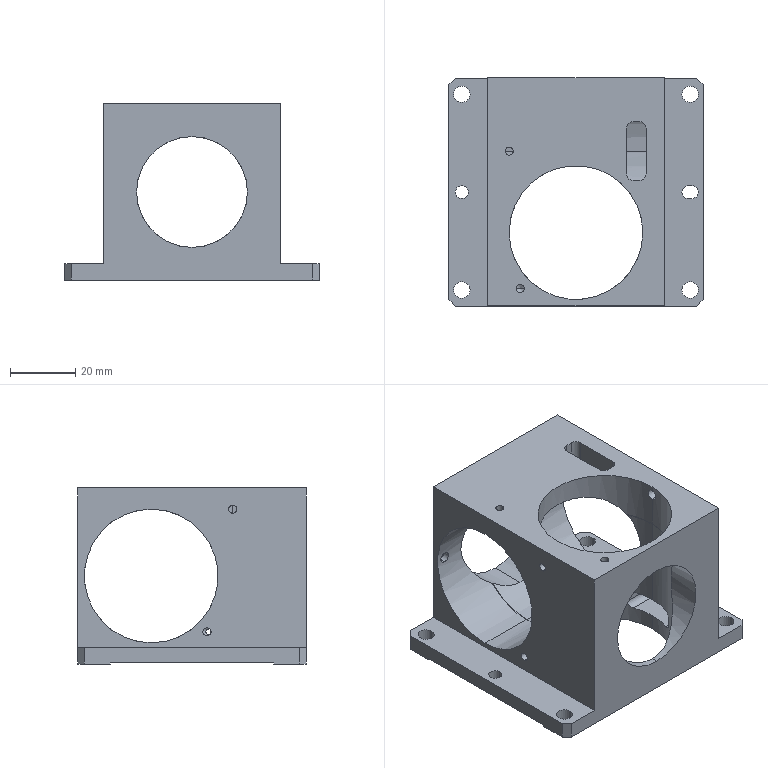NC program | NX | posted with a generic post | part box 78 x 70 x 54 mm
Whole program:
N10 G17 G21 G94 G90
(HOLE_MILLING_COPY , TOOL : D20)
N12 T02 M6
N14 G54
N16 G17 G0 G90 X0. Y0. B0. C0. S9500 M3
N18 G43 Z30. H2
N20 Z0.5
N22 G94 G3 X3.45 Y-3.45 R3.45 F1500.
N24 X6.9 Y0. R3.45
N26 X6.9 Y0. Z0. I-6.9 J0.
N28 X6.9 Y0. Z-0.5 I-6.9 J0.
N30 X6.9 Y0. Z-1. I-6.9 J0.
N32 X6.9 Y0. Z-1.5 I-6.9 J0.
N34 X6.9 Y0. Z-2. I-6.9 J0.
N36 X6.9 Y0. Z-2.5 I-6.9 J0.
N38 X6.9 Y0. Z-3. I-6.9 J0.
N40 X6.9 Y0. Z-3.5 I-6.9 J0.
N42 X6.9 Y0. Z-4. I-6.9 J0.
N44 X6.9 Y0. Z-4.5 I-6.9 J0.
N46 X6.9 Y0. Z-5. I-6.9 J0.
N48 X6.9 Y0. Z-5.5 I-6.9 J0.
N50 X6.9 Y0. Z-6. I-6.9 J0.
N52 X6.9 Y0. Z-6.5 I-6.9 J0.
N54 X6.9 Y0. Z-7. I-6.9 J0.
N56 X6.9 Y0. Z-7.5 I-6.9 J0.
N58 X6.9 Y0. Z-8. I-6.9 J0.
N60 X6.9 Y0. Z-8.5 I-6.9 J0.
N62 X6.9 Y0. Z-9. I-6.9 J0.
N64 X6.9 Y0. Z-9.5 I-6.9 J0.
N66 X6.9 Y0. Z-10. I-6.9 J0.
N68 X6.9 Y0. Z-10.5 I-6.9 J0.
N70 X6.9 Y0. Z-11. I-6.9 J0.
N72 X6.9 Y0. Z-11.5 I-6.9 J0.
N74 X6.9 Y0. Z-12. I-6.9 J0.
N76 X6.9 Y0. Z-12.5 I-6.9 J0.
N78 X6.9 Y0. Z-13. I-6.9 J0.
N80 X6.9 Y0. Z-13.5 I-6.9 J0.
N82 X6.9 Y0. Z-14. I-6.9 J0.
N84 X6.9 Y0. Z-14.5 I-6.9 J0.
N86 X6.9 Y0. Z-15. I-6.9 J0.
N88 X6.9 Y0. Z-15.5 I-6.9 J0.
N90 X6.9 Y0. Z-16. I-6.9 J0.
N92 X6.9 Y0. Z-16.5 I-6.9 J0.
N94 X6.9 Y0. Z-17. I-6.9 J0.
N96 X6.9 Y0. Z-17.5 I-6.9 J0.
N98 X6.9 Y0. Z-18. I-6.9 J0.
N100 X6.9 Y0. Z-18.5 I-6.9 J0.
N102 X6.9 Y0. Z-19. I-6.9 J0.
N104 X6.9 Y0. Z-19.5 I-6.9 J0.
N106 X6.9 Y0. Z-20. I-6.9 J0.
N108 X6.9 Y0. Z-20.5 I-6.9 J0.
N110 X6.9 Y0. Z-21. I-6.9 J0.
N112 X6.9 Y0. Z-21.5 I-6.9 J0.
N114 X6.9 Y0. Z-22. I-6.9 J0.
N116 X6.9 Y0. Z-22.5 I-6.9 J0.
N118 X6.9 Y0. Z-23. I-6.9 J0.
N120 X6.9 Y0. Z-23.5 I-6.9 J0.
N122 X6.9 Y0. Z-24. I-6.9 J0.
N124 X6.9 Y0. Z-24.5 I-6.9 J0.
N126 X6.9 Y0. Z-25. I-6.9 J0.
N128 X6.9 Y0. Z-25.5 I-6.9 J0.
N130 X6.9 Y0. Z-26. I-6.9 J0.
N132 X6.9 Y0. Z-26.5 I-6.9 J0.
N134 X6.9 Y0. Z-27. I-6.9 J0.
N136 X6.9 Y0. Z-27.5 I-6.9 J0.
N138 X6.9 Y0. Z-28. I-6.9 J0.
N140 X6.9 Y0. Z-28.5 I-6.9 J0.
N142 X6.9 Y0. Z-29. I-6.9 J0.
N144 X6.9 Y0. Z-29.5 I-6.9 J0.
N146 X6.9 Y0. Z-30. I-6.9 J0.
N148 X6.9 Y0. Z-30.5 I-6.9 J0.
N150 X6.9 Y0. Z-31. I-6.9 J0.
N152 X6.9 Y0. Z-31.5 I-6.9 J0.
N154 X6.9 Y0. Z-32. I-6.9 J0.
N156 X6.9 Y0. Z-32.5 I-6.9 J0.
N158 X6.9 Y0. Z-33. I-6.9 J0.
N160 X6.9 Y0. Z-33.5 I-6.9 J0.
N162 X6.9 Y0. Z-34. I-6.9 J0.
N164 X6.9 Y0. Z-34.5 I-6.9 J0.
N166 X6.9 Y0. Z-35. I-6.9 J0.
N168 X6.9 Y0. Z-35.5 I-6.9 J0.
N170 X6.9 Y0. Z-36. I-6.9 J0.
N172 X6.9 Y0. Z-36.5 I-6.9 J0.
N174 X6.9 Y0. Z-37. I-6.9 J0.
N176 X6.9 Y0. Z-37.5 I-6.9 J0.
N178 X6.9 Y0. Z-38. I-6.9 J0.
N180 X6.9 Y0. Z-38.5 I-6.9 J0.
N182 X6.9 Y0. Z-39. I-6.9 J0.
N184 X6.9 Y0. Z-39.5 I-6.9 J0.
N186 X6.9 Y0. Z-40. I-6.9 J0.
N188 X6.9 Y0. Z-40.5 I-6.9 J0.
N190 X6.9 Y0. Z-41. I-6.9 J0.
N192 X6.9 Y0. Z-41.5 I-6.9 J0.
N194 X6.9 Y0. Z-42. I-6.9 J0.
N196 X6.9 Y0. Z-42.5 I-6.9 J0.
N198 X6.9 Y0. Z-43. I-6.9 J0.
N200 X6.9 Y0. Z-43.5 I-6.9 J0.
N202 X6.9 Y0. Z-44. I-6.9 J0.
N204 X6.9 Y0. Z-44.5 I-6.9 J0.
N206 X6.9 Y0. Z-45. I-6.9 J0.
N208 X6.9 Y0. Z-45.5 I-6.9 J0.
N210 X6.9 Y0. Z-46. I-6.9 J0.
N212 X6.9 Y0. Z-46.5 I-6.9 J0.
N214 X6.9 Y0. Z-47. I-6.9 J0.
N216 X6.9 Y0. Z-47.5 I-6.9 J0.
N218 X6.9 Y0. Z-48. I-6.9 J0.
N220 X6.9 Y0. Z-48.5 I-6.9 J0.
N222 X6.9 Y0. Z-49. I-6.9 J0.
N224 X6.9 Y0. Z-49.5 I-6.9 J0.
N226 X6.9 Y0. Z-50. I-6.9 J0.
N228 X6.9 Y0. Z-50.5 I-6.9 J0.
N230 X6.9 Y0. Z-51. I-6.9 J0.
N232 X6.9 Y0. Z-51.5 I-6.9 J0.
N234 X6.9 Y0. Z-52. I-6.9 J0.
N236 X6.9 Y0. Z-52.5 I-6.9 J0.
N238 X6.9 Y0. Z-53. I-6.9 J0.
N240 X6.9 Y0. Z-53.5 I-6.9 J0.
N242 X6.9 Y0. Z-54. I-6.9 J0.
N244 X6.9 Y0. Z-54.5 I-6.9 J0.
N246 X6.9 Y0. Z-55. I-6.9 J0.
N248 X6.9 Y0. Z-55.5 I-6.9 J0.
N250 X6.9 Y0. Z-56. I-6.9 J0.
N252 X6.9 Y0. Z-56.5 I-6.9 J0.
N254 X6.9 Y0. Z-57. I-6.9 J0.
N256 X6.9 Y0. Z-57.5 I-6.9 J0.
N258 X6.9 Y0. Z-58. I-6.9 J0.
N260 X6.9 Y0. Z-58.5 I-6.9 J0.
N262 X6.9 Y0. Z-59. I-6.9 J0.
N264 X6.9 Y0. Z-59.5 I-6.9 J0.
N266 X6.9 Y0. Z-60. I-6.9 J0.
N268 X6.9 Y0. Z-60.5 I-6.9 J0.
N270 X6.9 Y0. Z-61. I-6.9 J0.
N272 X6.9 Y0. Z-61.5 I-6.9 J0.
N274 X6.9 Y0. Z-62. I-6.9 J0.
N276 X6.9 Y0. Z-62.5 I-6.9 J0.
N278 X6.9 Y0. Z-63. I-6.9 J0.
N280 X6.9 Y0. Z-63.5 I-6.9 J0.
N282 X6.9 Y0. Z-64. I-6.9 J0.
N284 X6.9 Y0. Z-64.5 I-6.9 J0.
N286 X6.9 Y0. Z-65. I-6.9 J0.
N288 X6.9 Y0. Z-65.5 I-6.9 J0.
N290 X6.9 Y0. Z-66. I-6.9 J0.
N292 X6.9 Y0. Z-66.5 I-6.9 J0.
N294 X6.9 Y0. Z-67. I-6.9 J0.
N296 X6.9 Y0. Z-67.5 I-6.9 J0.
N298 X6.9 Y0. Z-68. I-6.9 J0.
N300 X6.9 Y0. Z-68.5 I-6.9 J0.
N302 X6.9 Y0. Z-69. I-6.9 J0.
N304 X6.9 Y0. Z-69.5 I-6.9 J0.
N306 X6.9 Y0. Z-70. I-6.9 J0.
N308 X0. Y6.9 R6.9
N310 X6.9 Y0. R-6.9
N312 X3.45 Y3.45 R3.45
N314 X0. Y0. R3.45
N316 G0 Z30.
N318 M5
(11 , TOOL : D16JING)
N320 T13 M6
N322 G54
N324 G17 G0 G90 X0. Y0. B0. C0. S9500 M3
N326 G43 Z30. H13
N328 Z0.5
N330 G94 G1 X5.41 Y-2.353 F1000.
N332 G3 X9. Y0. R2.566
N334 X9. Y0. Z-9.5 I-9. J0.
N336 X9. Y0. Z-19.5 I-9. J0.
N338 X9. Y0. Z-29.5 I-9. J0.
N340 X9. Y0. Z-39.5 I-9. J0.
N342 X9. Y0. Z-49.5 I-9. J0.
N344 X9. Y0. Z-59.5 I-9. J0.
N346 X9. Y0. Z-69.5 I-9. J0.
N348 X8.56 Y2.781 Z-70. R9.
N350 X-2.781 Y8.56 R9.
N352 X8.56 Y2.781 R-9.
N354 X4.418 Y3.91 R2.566
N356 G1 X0. Y0.
N358 G0 Z30.
N360 M5
(DRILLING_1_COPY_1 , TOOL : D6A45)
N362 T07 M6
N364 G54
N366 G17 G0 G90 X-24. Y0. B0. C0. S5000 M3
N368 G43 Z30. H7
N370 G94 G81 G98 Z-1.1 F250. R3.
N372 G80
N374 G0 X-24. Y0. Z30.
N376 M5
(DRILLING_1_COPY_1_COPY , TOOL : 3.3ZT)
N378 T03 M6
N380 G54
N382 G17 G0 G90 X-24. Y0. B0. C0. S2000 M3
N384 G43 Z30. H3
N386 G94 G83 G98 Z-4.558 F150. Q2. R3.
N388 G80
N390 G0 X-24. Y0. Z30.
N392 M5
(PLANAR_MILL_COPY_1_1_COPY_COPY_1 , TOOL : D6A45)
N394 T07 M6
N396 G54
N398 G17 G0 G90 X-24.626 Y-0.424 B0. C0. S9500 M3
N400 G43 Z30. H7
N402 Z0.5
N404 G94 G1 X-24.552 Y-0.552 Z0.46 F1250.
N406 X-24.214 Y-0.75 Z0.356
N408 X-23.786 Z0.241
N410 X-23.448 Y-0.552 Z0.136
N412 X-23.25 Y-0.214 Z0.031
N414 Y0.214 Z-0.084
N416 X-23.448 Y0.552 Z-0.189
N418 X-23.786 Y0.75 Z-0.294
N420 X-24.214 Z-0.408
N422 X-24.552 Y0.552 Z-0.513
N424 X-24.75 Y0.214 Z-0.618
N426 Y-0.214 Z-0.733
N428 X-24.552 Y-0.552 Z-0.838
N430 X-24.214 Y-0.75 Z-0.943
N432 X-24. Z-1.
N434 G3 X-23.25 Y0. R0.75
N436 X-24. Y-0.75 R-0.75
N438 X-23.567 Y-0.5 R0.5
N440 G1 Z0.5
N442 G0 Z30.
N444 X-1.303 Y-14.843
N446 Z0.5
N448 G1 Z-1.
N450 X-0.866 Y-15.6
N452 G3 X0. Y-16.1 R1.
N454 X16.1 Y0. R16.1
N456 X0. Y-16.1 R-16.1
N458 X0.866 Y-15.6 R1.
N460 G1 X1.303 Y-14.843
N462 Z0.5
N464 G0 Z30.
N466 M5
N468 M2